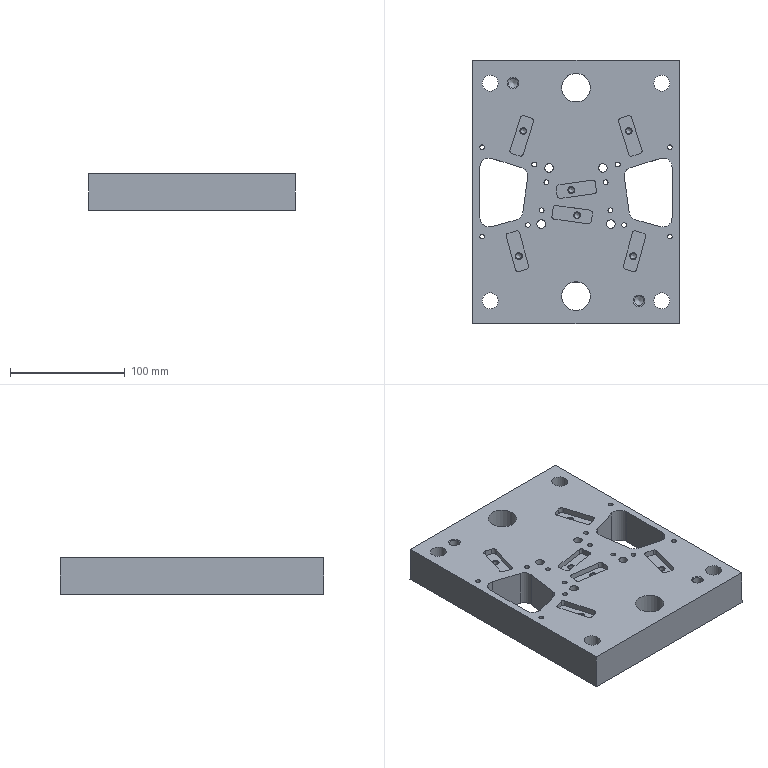Part | STEP file | gslz 2016.10.28-6_id22_x_t | 1 solid | 182 faces | box 180 x 230 x 32 mm | volume 1103435 mm3 | cylinder 72 | plane 60 | cone 40 | spline 8 | other 2 | commonest cylinder face diameters 4.1 x12 6 x12 6.5 x12 4 x10 5 x10 7.5 x4